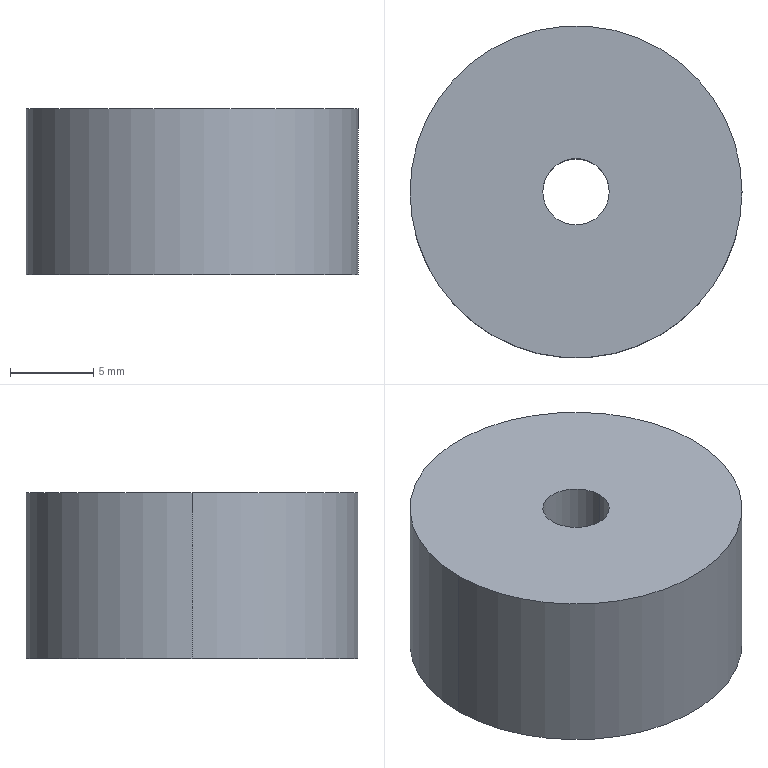Part | STEP file | Foot pad | 1 solid | 6 faces | box 20 x 20 x 10 mm | volume 3016 mm3 | cylinder 4 | plane 2 | commonest cylinder face diameters 4 x2 20 x2
STEP:
#1=CARTESIAN_POINT('',(-10.,0.,10.));
#2=VERTEX_POINT('',#1);
#3=CARTESIAN_POINT('',(10.,0.,10.));
#4=VERTEX_POINT('',#3);
#5=CARTESIAN_POINT('',(0.,0.,10.));
#6=DIRECTION('',(0.,0.,-1.));
#7=DIRECTION('',(-1.,0.,0.));
#8=AXIS2_PLACEMENT_3D('',#5,#6,#7);
#9=CIRCLE('',#8,10.);
#10=EDGE_CURVE('',#2,#4,#9,.T.);
#11=ORIENTED_EDGE('',*,*,#10,.T.);
#12=CARTESIAN_POINT('',(10.,0.,0.));
#13=VERTEX_POINT('',#12);
#14=CARTESIAN_POINT('',(10.,0.,10.));
#15=DIRECTION('',(0.,0.,-1.));
#16=VECTOR('',#15,1000.);
#17=LINE('',#14,#16);
#18=EDGE_CURVE('',#4,#13,#17,.T.);
#19=ORIENTED_EDGE('',*,*,#18,.T.);
#20=CARTESIAN_POINT('',(-10.,0.,0.));
#21=VERTEX_POINT('',#20);
#22=CARTESIAN_POINT('',(0.,0.,0.));
#23=DIRECTION('',(0.,0.,1.));
#24=DIRECTION('',(-1.,0.,0.));
#25=AXIS2_PLACEMENT_3D('',#22,#23,#24);
#26=CIRCLE('',#25,10.);
#27=EDGE_CURVE('',#13,#21,#26,.T.);
#28=ORIENTED_EDGE('',*,*,#27,.T.);
#29=CARTESIAN_POINT('',(-10.,0.,10.));
#30=DIRECTION('',(0.,0.,-1.));
#31=VECTOR('',#30,1000.);
#32=LINE('',#29,#31);
#33=EDGE_CURVE('',#2,#21,#32,.T.);
#34=ORIENTED_EDGE('',*,*,#33,.F.);
#35=EDGE_LOOP('',(#11,#19,#28,#34));
#36=FACE_OUTER_BOUND('',#35,.T.);
#37=CARTESIAN_POINT('',(0.,0.,10.));
#38=DIRECTION('',(0.,0.,-1.));
#39=DIRECTION('',(-1.,0.,0.));
#40=AXIS2_PLACEMENT_3D('',#37,#38,#39);
#41=CYLINDRICAL_SURFACE('',#40,10.);
#42=ADVANCED_FACE('',(#36),#41,.T.);
#43=CARTESIAN_POINT('',(2.,0.,10.));
#44=VERTEX_POINT('',#43);
#45=CARTESIAN_POINT('',(-2.,0.,10.));
#46=VERTEX_POINT('',#45);
#47=CARTESIAN_POINT('',(0.,0.,10.));
#48=DIRECTION('',(0.,0.,-1.));
#49=DIRECTION('',(-1.,0.,0.));
#50=AXIS2_PLACEMENT_3D('',#47,#48,#49);
#51=CIRCLE('',#50,2.);
#52=EDGE_CURVE('',#44,#46,#51,.T.);
#53=ORIENTED_EDGE('',*,*,#52,.F.);
#54=CARTESIAN_POINT('',(2.,0.,0.));
#55=VERTEX_POINT('',#54);
#56=CARTESIAN_POINT('',(2.,0.,10.));
#57=DIRECTION('',(0.,0.,-1.));
#58=VECTOR('',#57,1000.);
#59=LINE('',#56,#58);
#60=EDGE_CURVE('',#44,#55,#59,.T.);
#61=ORIENTED_EDGE('',*,*,#60,.T.);
#62=CARTESIAN_POINT('',(-2.,0.,0.));
#63=VERTEX_POINT('',#62);
#64=CARTESIAN_POINT('',(0.,0.,0.));
#65=DIRECTION('',(0.,0.,-1.));
#66=DIRECTION('',(-1.,0.,0.));
#67=AXIS2_PLACEMENT_3D('',#64,#65,#66);
#68=CIRCLE('',#67,2.);
#69=EDGE_CURVE('',#55,#63,#68,.T.);
#70=ORIENTED_EDGE('',*,*,#69,.T.);
#71=CARTESIAN_POINT('',(-2.,0.,10.));
#72=DIRECTION('',(0.,0.,-1.));
#73=VECTOR('',#72,1000.);
#74=LINE('',#71,#73);
#75=EDGE_CURVE('',#46,#63,#74,.T.);
#76=ORIENTED_EDGE('',*,*,#75,.F.);
#77=EDGE_LOOP('',(#53,#61,#70,#76));
#78=FACE_OUTER_BOUND('',#77,.T.);
#79=CARTESIAN_POINT('',(0.,0.,10.));
#80=DIRECTION('',(0.,0.,-1.));
#81=DIRECTION('',(-1.,0.,0.));
#82=AXIS2_PLACEMENT_3D('',#79,#80,#81);
#83=CYLINDRICAL_SURFACE('',#82,2.);
#84=ADVANCED_FACE('',(#78),#83,.F.);
#85=ORIENTED_EDGE('',*,*,#18,.F.);
#86=CARTESIAN_POINT('',(0.,0.,10.));
#87=DIRECTION('',(0.,0.,-1.));
#88=DIRECTION('',(-1.,0.,0.));
#89=AXIS2_PLACEMENT_3D('',#86,#87,#88);
#90=CIRCLE('',#89,10.);
#91=EDGE_CURVE('',#4,#2,#90,.T.);
#92=ORIENTED_EDGE('',*,*,#91,.T.);
#93=ORIENTED_EDGE('',*,*,#33,.T.);
#94=CARTESIAN_POINT('',(0.,0.,0.));
#95=DIRECTION('',(0.,0.,1.));
#96=DIRECTION('',(-1.,0.,0.));
#97=AXIS2_PLACEMENT_3D('',#94,#95,#96);
#98=CIRCLE('',#97,10.);
#99=EDGE_CURVE('',#21,#13,#98,.T.);
#100=ORIENTED_EDGE('',*,*,#99,.T.);
#101=EDGE_LOOP('',(#85,#92,#93,#100));
#102=FACE_OUTER_BOUND('',#101,.T.);
#103=CARTESIAN_POINT('',(0.,0.,10.));
#104=DIRECTION('',(0.,0.,-1.));
#105=DIRECTION('',(-1.,0.,0.));
#106=AXIS2_PLACEMENT_3D('',#103,#104,#105);
#107=CYLINDRICAL_SURFACE('',#106,10.);
#108=ADVANCED_FACE('',(#102),#107,.T.);
#109=ORIENTED_EDGE('',*,*,#99,.F.);
#110=ORIENTED_EDGE('',*,*,#27,.F.);
#111=EDGE_LOOP('',(#109,#110));
#112=FACE_OUTER_BOUND('',#111,.T.);
#113=CARTESIAN_POINT('',(0.,0.,0.));
#114=DIRECTION('',(0.,0.,-1.));
#115=DIRECTION('',(-1.,0.,0.));
#116=AXIS2_PLACEMENT_3D('',#113,#114,#115);
#117=CIRCLE('',#116,2.);
#118=EDGE_CURVE('',#63,#55,#117,.T.);
#119=ORIENTED_EDGE('',*,*,#118,.F.);
#120=ORIENTED_EDGE('',*,*,#69,.F.);
#121=EDGE_LOOP('',(#119,#120));
#122=FACE_BOUND('',#121,.T.);
#123=CARTESIAN_POINT('',(0.,0.,0.));
#124=DIRECTION('',(0.,0.,1.));
#125=DIRECTION('',(1.,0.,0.));
#126=AXIS2_PLACEMENT_3D('',#123,#124,#125);
#127=PLANE('',#126);
#128=ADVANCED_FACE('',(#112,#122),#127,.F.);
#129=ORIENTED_EDGE('',*,*,#10,.F.);
#130=ORIENTED_EDGE('',*,*,#91,.F.);
#131=EDGE_LOOP('',(#129,#130));
#132=FACE_OUTER_BOUND('',#131,.T.);
#133=CARTESIAN_POINT('',(0.,0.,10.));
#134=DIRECTION('',(0.,0.,-1.));
#135=DIRECTION('',(-1.,0.,0.));
#136=AXIS2_PLACEMENT_3D('',#133,#134,#135);
#137=CIRCLE('',#136,2.);
#138=EDGE_CURVE('',#46,#44,#137,.T.);
#139=ORIENTED_EDGE('',*,*,#138,.T.);
#140=ORIENTED_EDGE('',*,*,#52,.T.);
#141=EDGE_LOOP('',(#139,#140));
#142=FACE_BOUND('',#141,.T.);
#143=CARTESIAN_POINT('',(0.,0.,10.));
#144=DIRECTION('',(0.,0.,1.));
#145=DIRECTION('',(1.,0.,0.));
#146=AXIS2_PLACEMENT_3D('',#143,#144,#145);
#147=PLANE('',#146);
#148=ADVANCED_FACE('',(#132,#142),#147,.T.);
#149=ORIENTED_EDGE('',*,*,#60,.F.);
#150=ORIENTED_EDGE('',*,*,#138,.F.);
#151=ORIENTED_EDGE('',*,*,#75,.T.);
#152=ORIENTED_EDGE('',*,*,#118,.T.);
#153=EDGE_LOOP('',(#149,#150,#151,#152));
#154=FACE_OUTER_BOUND('',#153,.T.);
#155=CARTESIAN_POINT('',(0.,0.,10.));
#156=DIRECTION('',(0.,0.,-1.));
#157=DIRECTION('',(-1.,0.,0.));
#158=AXIS2_PLACEMENT_3D('',#155,#156,#157);
#159=CYLINDRICAL_SURFACE('',#158,2.);
#160=ADVANCED_FACE('',(#154),#159,.F.);
#161=CLOSED_SHELL('',(#42,#84,#108,#128,#148,#160));
#162=MANIFOLD_SOLID_BREP('',#161);
#163=CARTESIAN_POINT('',(0.,0.,0.));
#164=DIRECTION('',(0.,0.,1.));
#165=DIRECTION('',(1.,0.,0.));
#166=AXIS2_PLACEMENT_3D('',#163,#164,#165);
#167=(LENGTH_UNIT()NAMED_UNIT(*)SI_UNIT(.MILLI.,.METRE.));
#168=UNCERTAINTY_MEASURE_WITH_UNIT(LENGTH_MEASURE(0.00001),#167,'','');
#169=(NAMED_UNIT(*)PLANE_ANGLE_UNIT()SI_UNIT($,.RADIAN.));
#170=(NAMED_UNIT(*)SI_UNIT($,.STERADIAN.)SOLID_ANGLE_UNIT());
#171=(GEOMETRIC_REPRESENTATION_CONTEXT(3)GLOBAL_UNCERTAINTY_ASSIGNED_CONTEXT((#168))GLOBAL_UNIT_ASSIGNED_CONTEXT((#167,#169,#170))REPRESENTATION_CONTEXT('',''));
#172=ADVANCED_BREP_SHAPE_REPRESENTATION('',(#162,#166),#171);